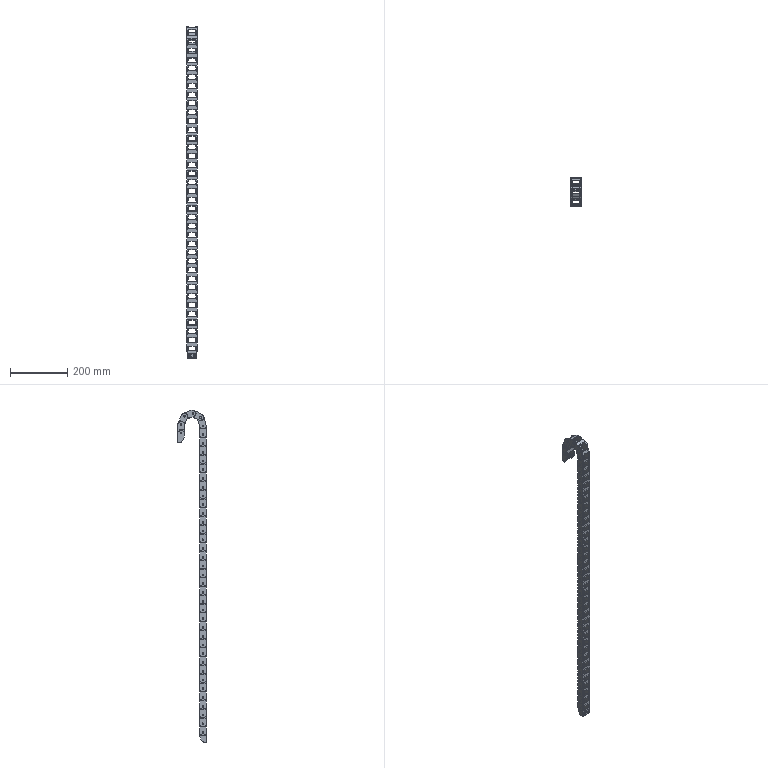Part | SolidWorks | 42 solids | 2617 faces | box 36.5 x 99.183 x 1156 mm | volume 350989 mm3 | plane 1354 | cylinder 1251 | cone 8 | torus 4 | commonest cylinder face diameters 1 x420 6 x324 5.9 x160 16.02 x80 18.716 x80 19.5 x80